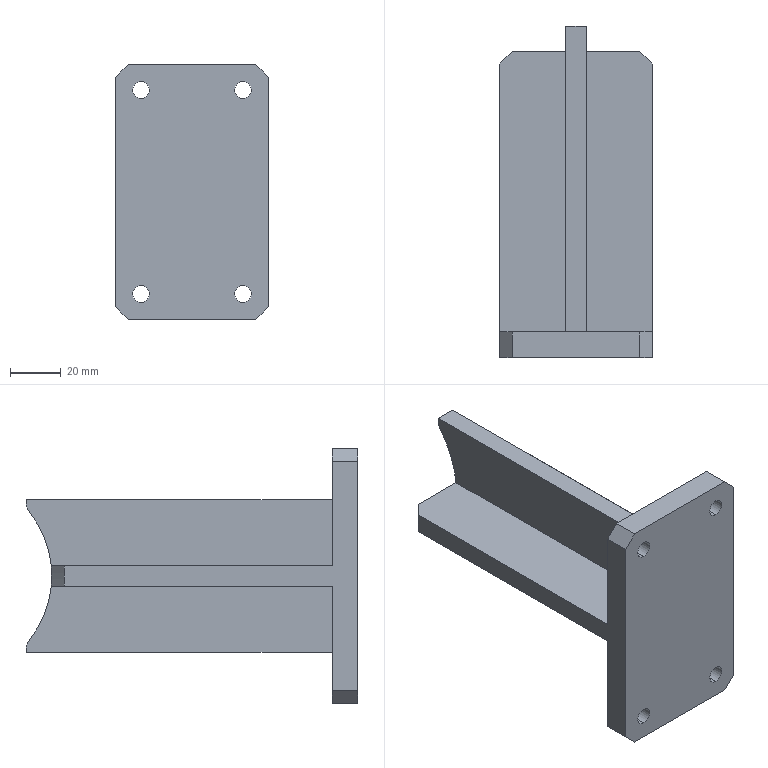Part | STEP file | Tube support base-rear end | 1 solid | 36 faces | box 60 x 130 x 100 mm | volume 158412 mm3 | plane 23 | cylinder 11 | cone 2 | commonest cylinder face diameters 6.6 x8 10 x2 80 x1